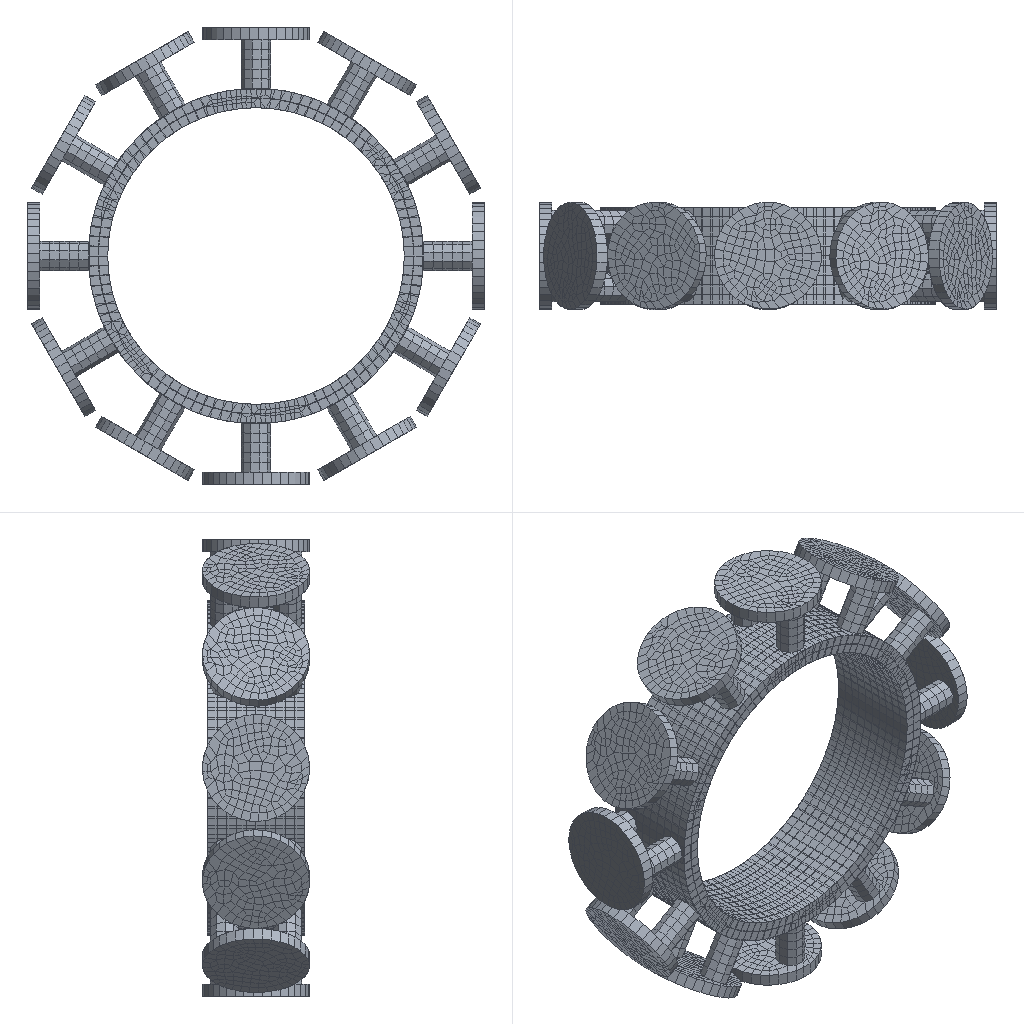Simulation study | abaqus
Set-up summary:
category,name,step,type,value,unit,region
solver,abaqus
solver,version,,,Abaqus/Standard 2020
units,not stated in the deck,,not stated
analysis,deck,,static,static
load_step,Step-1,Step-1,static
load_step,requested,,,1
mesh,nodes,,,21948
mesh,elements,,,16928
element_type,S4R,,shell,11811
element_type,C3D8R,,solid,5117
load,load commands in deck,,count,12
bc,support commands in deck,,count,5
material,CON,,in results
material,FRP,,in results
material,MATERIAL-3,,in results
check,setup vs results,,match,"per instance, exact: element labels, types and connectivity; labels of the nodes the elements use; coordinates of those nodes at SINGLE_PRECISION in 18 of 19 instance(s)"
Abaqus input file, long lists of numbers shortened:
*Heading
** Job name: Job-2 Model name: Model-1-Copy2
** Generated by: Abaqus/CAE 2020
*Preprint, echo=NO, model=NO, history=NO, contact=NO
**
** PARTS
**
*Part, name=con
*Node
      1,         610.,   1219.589,           0.
      2,         650.,   1219.589,           0.
** (916 more lines like these left out)
*Element, type=C3D8R
  1,  10,  11,  14,  13,   1,   2,   5,   4
  2,  11,  12,  15,  14,   2,   3,   6,   5
** (406 more lines like these left out)
*Nset, nset=Set-1, generate
   1,  918,    1
*Elset, elset=Set-1, generate
   1,  408,    1
** Section: con
*Solid Section, elset=Set-1, material=con
,
*End Part
**
*Part, name=frp
*Node
      1,   666.024,    1000.002,           0.
      2,   666.024,    1160.002,           0.
** (8318 more lines like these left out)
*Element, type=S4R
   1,   48,   41,    6,    1
   2,   41,   42,    7,    6
** (8318 more lines like these left out)
*Nset, nset=Set-3, generate
    1,  8320,     1
*Elset, elset=Set-3, generate
    1,  8320,     1
** Section: Section-1
*Shell Section, elset=Set-3, material=frp
7., 5
*End Part
**
*Part, name=gangban
*Node
      1,         610.,   1059.589,           0.
      2,         610.,   979.589,           0.
** (3081 more lines like these left out)
*Element, type=S4R
  1,    1,   13, 1241,  108
  2,   13,   14, 1242, 1241
** (3489 more lines like these left out)
*Nset, nset=Set-3, generate
    1,  3083,     1
*Elset, elset=Set-3, generate
    1,  3491,     1
** Section: Section-1
*Shell Section, elset=Set-3, material=frp
7., 5
*End Part
**
*Part, name=m1
*Node
      1,         890.,   1007.07,  -46.852
      2,   688.407,   1007.07,  -46.852
** (478 more lines like these left out)
*Element, type=C3D8R
 1, 434, 437, 435, 433, 114, 117, 115, 113
 2, 438, 434, 433, 436, 118, 114, 113, 116
** (239 more lines like these left out)
*Nset, nset=Set-1, generate
   1,  480,    1
*Elset, elset=Set-1, generate
   1,  241,    1
** Section: m
*Solid Section, elset=Set-1, material=Material-3
,
*End Part
**
*Part, name=m2
*Node
      1,   747.337,   1007.07,  -485.575
      2,   572.752,   1007.07,   -384.779
** (516 more lines like these left out)
*Element, type=C3D8R
 1, 119,  12,  11, 120, 453, 130, 129, 454
 2, 114,  10,   9, 121, 448, 128, 127, 455
** (273 more lines like these left out)
*Nset, nset=Set-3, generate
   1,  518,    1
*Elset, elset=Set-3, generate
   1,  275,    1
** Section: m
*Solid Section, elset=Set-3, material=Material-3
,
*End Part
**
*Part, name=m3
*Node
      1,   404.425,   1007.07,   -794.189
      2,   303.629,   1007.07,  -619.604
** (537 more lines like these left out)
*Element, type=C3D8R
 1, 119,  12,  11, 120, 462, 130, 129, 463
 2, 114,  10,   9, 121, 457, 128, 127, 464
** (291 more lines like these left out)
*Nset, nset=Set-1, generate
   1,  539,    1
*Elset, elset=Set-1, generate
   1,  293,    1
** Section: m
*Solid Section, elset=Set-1, material=Material-3
,
*End Part
**
*Part, name=m4
*Node
      1,  -46.852,   1007.07,        -890.
      2,  -46.852,   1007.07,  -688.407
** (478 more lines like these left out)
*Element, type=C3D8R
 1, 434, 437, 435, 433, 114, 117, 115, 113
 2, 438, 434, 433, 436, 118, 114, 113, 116
** (239 more lines like these left out)
*Nset, nset=Set-1, generate
   1,  480,    1
*Elset, elset=Set-1, generate
   1,  241,    1
** Section: m
*Solid Section, elset=Set-1, material=Material-3
,
*End Part
**
*Part, name=m5
*Node
      1,  -485.575,   1007.07,  -747.337
      2,   -384.779,   1007.07,  -572.752
** (487 more lines like these left out)
*Element, type=C3D8R
 1, 430, 123, 124, 434, 113,   8,   9, 117
 2, 432, 437, 433, 431, 115, 120, 116, 114
** (251 more lines like these left out)
*Nset, nset=Set-1, generate
   1,  489,    1
*Elset, elset=Set-1, generate
   1,  253,    1
** Section: m
*Solid Section, elset=Set-1, material=Material-3
,
*End Part
**
*Part, name=m6
*Node
      1,   -794.189,   1007.07,  -404.425
      2,  -619.604,   1007.07,  -303.629
** (466 more lines like these left out)
*Element, type=C3D8R
 1, 429, 118, 119, 120, 113,   8,   9,  10
 2, 125, 431, 430, 124,  15, 115, 114,  14
** (228 more lines like these left out)
*Nset, nset=Set-1, generate
   1,  468,    1
*Elset, elset=Set-1, generate
   1,  230,    1
** Section: m
*Solid Section, elset=Set-1, material=Material-3
,
*End Part
**
*Part, name=m7
*Node
      1,        -890.,   1007.07,   46.852
      2,  -688.407,   1007.07,   46.852
** (462 more lines like these left out)
*Element, type=C3D8R
 1, 118, 119, 427, 425,   8,   9, 115, 113
 2, 428, 426, 425, 427, 116, 114, 113, 115
** (226 more lines like these left out)
*Nset, nset=Set-1, generate
   1,  464,    1
*Elset, elset=Set-1, generate
   1,  228,    1
** Section: m
*Solid Section, elset=Set-1, material=Material-3
,
*End Part
**
*Part, name=m8
*Node
      1,  -747.337,   1007.07,   485.575
      2,  -572.752,   1007.07,    384.779
** (516 more lines like these left out)
*Element, type=C3D8R
 1, 119,  12,  11, 120, 453, 130, 129, 454
 2,  10,   9, 121, 114, 128, 127, 455, 448
** (273 more lines like these left out)
*Nset, nset=Set-1, generate
   1,  518,    1
*Elset, elset=Set-1, generate
   1,  275,    1
** Section: m
*Solid Section, elset=Set-1, material=Material-3
,
*End Part
**
*Part, name=m9
*Node
      1,  -404.425,   1007.07,    794.189
      2,  -303.629,   1007.07,   619.604
** (468 more lines like these left out)
*Element, type=C3D8R
 1, 423, 120, 121, 426, 113,   8,   9, 116
 2, 428, 426, 123, 124, 118, 116,  11,  12
** (234 more lines like these left out)
*Nset, nset=Set-1, generate
   1,  470,    1
*Elset, elset=Set-1, generate
   1,  236,    1
** Section: m
*Solid Section, elset=Set-1, material=Material-3
,
*End Part
**
*Part, name=m10
*Node
      1,   46.852,   1007.07,         890.
      2,   46.852,   1007.07,   688.407
** (541 more lines like these left out)
*Element, type=C3D8R
 1, 113, 123, 119, 120, 460, 470, 466, 467
 2, 114,  10,   9, 121, 461, 128, 127, 468
** (293 more lines like these left out)
*Nset, nset=Set-1, generate
   1,  543,    1
*Elset, elset=Set-1, generate
   1,  295,    1
** Section: m
*Solid Section, elset=Set-1, material=Material-3
,
*End Part
**
*Part, name=m11
*Node
      1,   485.575,   1007.07,   747.337
      2,    384.779,   1007.07,   572.752
** (516 more lines like these left out)
*Element, type=C3D8R
 1, 119,  12,  11, 120, 453, 130, 129, 454
 2, 114,  10,   9, 121, 448, 128, 127, 455
** (273 more lines like these left out)
*Nset, nset=Set-1, generate
   1,  518,    1
*Elset, elset=Set-1, generate
   1,  275,    1
** Section: m
*Solid Section, elset=Set-1, material=Material-3
,
*End Part
**
*Part, name=m12
*Node
      1,    794.189,   1007.07,   404.425
      2,   619.604,   1007.07,   303.629
** (466 more lines like these left out)
*Element, type=C3D8R
 1, 421, 120, 121, 424, 113,   8,   9, 116
 2, 426, 424, 123, 124, 118, 116,  11,  12
** (233 more lines like these left out)
*Nset, nset=Set-1, generate
   1,  468,    1
*Elset, elset=Set-1, generate
   1,  235,    1
** Section: m
*Solid Section, elset=Set-1, material=Material-3
,
*End Part
**
**
** ASSEMBLY
**
*Assembly, name=Assembly
**
*Instance, name=con-1, part=con
*End Instance
**
*Instance, name=frp-1, part=frp
*End Instance
**
*Instance, name=gangban-1, part=gangban
*End Instance
**
*Instance, name=con-1-lin-1-2, part=con
          0.,         -80.,           0.
*End Instance
**
*Instance, name=con-1-lin-1-3, part=con
          0.,        -160.,           0.
*End Instance
**
*Instance, name=con-1-lin-1-4, part=con
          0.,        -240.,           0.
*End Instance
**
*Instance, name=con-1-lin-1-5, part=con
          0.,        -320.,           0.
*End Instance
**
*Instance, name=m1-1, part=m1
*End Instance
**
*Instance, name=m2-1, part=m2
*End Instance
**
*Instance, name=m3-1, part=m3
*End Instance
**
*Instance, name=m4-1, part=m4
*End Instance
**
*Instance, name=m5-1, part=m5
*End Instance
**
*Instance, name=m6-1, part=m6
*End Instance
**
*Instance, name=m7-1, part=m7
*End Instance
**
*Instance, name=m8-1, part=m8
*End Instance
**
*Instance, name=m9-1, part=m9
*End Instance
**
*Instance, name=m10-1, part=m10
*End Instance
**
*Instance, name=m11-1, part=m11
*End Instance
**
*Instance, name=m12-1, part=m12
*End Instance
**
*Node
      1,         470.,   1099.589,   814.064
*Node
      2,   814.064,   1099.589,         470.
*Node
      3,         940.,   1099.589, 1.34711146e-14
*Node
      4,   814.064,   1099.589,        -470.
*Node
      5,         470.,   1099.589,  -814.064
*Node
      6, 7.10295131e-14,   1099.589,        -940.
*Node
      7,        -470.,   1099.589,  -814.064
*Node
      8,  -814.064,   1099.589,        -470.
*Node
      9,        -940.,   1099.589, -1.28587909e-13
*Node
     10,  -814.064,   1099.589,         470.
*Node
     11,        -470.,   1099.589,   814.064
*Node
     12, -1.86146319e-13,   1099.589,         940.
*Node
     13,           0.,   1059.589, -3.73517271e-14
*Nset, nset=Set-3, instance=con-1
   7,   8,   9,  16,  17,  18,  25,  26,  27,  34,  35,  36,  43,  44,  45,  52
  53,  54,  61,  62,  63,  70,  71,  72,  79,  80,  81,  88,  89,  90,  97,  98
** (18 more lines like these left out)
*Elset, elset=Set-3, instance=con-1
   3,   4,   7,   8,  11,  12,  15,  16,  19,  20,  23,  24,  27,  28,  31,  32
  35,  36,  39,  40,  43,  44,  47,  48,  51,  52,  55,  56,  59,  60,  63,  64
** (11 more lines like these left out)
*Nset, nset=Set-4, instance=m1-1
   4,   5,  34,  35,  36,  37,  38,  39,  40,  41,  42,  43,  44,  45,  46,  47
  48,  49,  50,  51,  52,  53,  54,  55,  56,  57,  58,  59,  60,  61,  62,  63
** (3 more lines like these left out)
*Nset, nset=Set-4, instance=m2-1
   4,   5,  34,  35,  36,  37,  38,  39,  40,  41,  42,  43,  44,  45,  46,  47
  48,  49,  50,  51,  52,  53,  54,  55,  56,  57,  58,  59,  60,  61,  62,  63
** (3 more lines like these left out)
*Nset, nset=Set-4, instance=m4-1
   4,   5,  34,  35,  36,  37,  38,  39,  40,  41,  42,  43,  44,  45,  46,  47
  48,  49,  50,  51,  52,  53,  54,  55,  56,  57,  58,  59,  60,  61,  62,  63
** (3 more lines like these left out)
*Nset, nset=Set-4, instance=m6-1
   4,   5,  34,  35,  36,  37,  38,  39,  40,  41,  42,  43,  44,  45,  46,  47
  48,  49,  50,  51,  52,  53,  54,  55,  56,  57,  58,  59,  60,  61,  62,  63
** (3 more lines like these left out)
*Nset, nset=Set-4, instance=m10-1
   4,   5,  34,  35,  36,  37,  38,  39,  40,  41,  42,  43,  44,  45,  46,  47
  48,  49,  50,  51,  52,  53,  54,  55,  56,  57,  58,  59,  60,  61,  62,  63
** (3 more lines like these left out)
*Nset, nset=Set-4, instance=m8-1
   4,   5,  34,  35,  36,  37,  38,  39,  40,  41,  42,  43,  44,  45,  46,  47
  48,  49,  50,  51,  52,  53,  54,  55,  56,  57,  58,  59,  60,  61,  62,  63
** (3 more lines like these left out)
*Nset, nset=Set-4, instance=m12-1
   4,   5,  34,  35,  36,  37,  38,  39,  40,  41,  42,  43,  44,  45,  46,  47
  48,  49,  50,  51,  52,  53,  54,  55,  56,  57,  58,  59,  60,  61,  62,  63
** (3 more lines like these left out)
*Nset, nset=Set-4, instance=m3-1
   4,   5,  34,  35,  36,  37,  38,  39,  40,  41,  42,  43,  44,  45,  46,  47
  48,  49,  50,  51,  52,  53,  54,  55,  56,  57,  58,  59,  60,  61,  62,  63
** (3 more lines like these left out)
*Nset, nset=Set-4, instance=m7-1
   4,   5,  34,  35,  36,  37,  38,  39,  40,  41,  42,  43,  44,  45,  46,  47
  48,  49,  50,  51,  52,  53,  54,  55,  56,  57,  58,  59,  60,  61,  62,  63
** (3 more lines like these left out)
*Nset, nset=Set-4, instance=m11-1
   4,   5,  34,  35,  36,  37,  38,  39,  40,  41,  42,  43,  44,  45,  46,  47
  48,  49,  50,  51,  52,  53,  54,  55,  56,  57,  58,  59,  60,  61,  62,  63
** (3 more lines like these left out)
*Nset, nset=Set-4, instance=m5-1
   4,   5,  34,  35,  36,  37,  38,  39,  40,  41,  42,  43,  44,  45,  46,  47
  48,  49,  50,  51,  52,  53,  54,  55,  56,  57,  58,  59,  60,  61,  62,  63
** (3 more lines like these left out)
*Nset, nset=Set-4, instance=m9-1
   4,   5,  34,  35,  36,  37,  38,  39,  40,  41,  42,  43,  44,  45,  46,  47
  48,  49,  50,  51,  52,  53,  54,  55,  56,  57,  58,  59,  60,  61,  62,  63
** (3 more lines like these left out)
*Elset, elset=Set-4, instance=m1-1
  77,  80,  82,  83,  84,  86,  88,  90,  91,  92,  98,  99, 100, 104, 105, 106
 107, 109, 111, 112, 113, 116, 118, 122, 129, 130, 131, 132, 133, 134, 136, 137
** (1 more lines like these left out)
*Elset, elset=Set-4, instance=m2-1
 101, 106, 107, 108, 109, 110, 111, 112, 113, 115, 117, 122, 123, 130, 131, 132
 133, 134, 138, 141, 143, 147, 153, 154, 156, 157, 158, 159, 160, 161, 164, 165
** (1 more lines like these left out)
*Elset, elset=Set-4, instance=m4-1
  77,  80,  82,  83,  84,  87,  89,  91,  92,  93,  99, 100, 101, 104, 105, 106
 107, 109, 111, 112, 113, 116, 117, 121, 129, 130, 131, 132, 133, 134, 136, 137
** (1 more lines like these left out)
*Elset, elset=Set-4, instance=m6-1
  52,  53,  61,  62,  66,  67,  68,  70,  71,  72,  73,  74,  76,  80,  84,  88
  89,  92,  93,  94,  97, 101, 107, 112, 113, 114, 117, 118, 119, 121, 122, 124
** (1 more lines like these left out)
*Elset, elset=Set-4, instance=m10-1
 103, 111, 112, 114, 115, 116, 118, 120, 123, 124, 126, 131, 133, 137, 138, 139
 140, 142, 145, 148, 150, 153, 160, 161, 162, 163, 164, 165, 166, 167, 168, 170
** (1 more lines like these left out)
*Elset, elset=Set-4, instance=m8-1
 100, 105, 106, 107, 108, 109, 110, 111, 112, 113, 115, 120, 121, 122, 130, 131
 133, 134, 138, 142, 145, 153, 154, 155, 156, 157, 158, 159, 161, 162, 165, 166
** (1 more lines like these left out)
*Elset, elset=Set-4, instance=m12-1
  62,  63,  71,  75,  76,  77,  79,  80,  81,  82,  83,  85,  89,  91,  94,  97
  98, 101, 102, 103, 106, 110, 115, 122, 123, 124, 125, 126, 129, 130, 134, 135
** (1 more lines like these left out)
*Elset, elset=Set-4, instance=m3-1
  95,  96, 104, 109, 110, 111, 113, 114, 115, 116, 118, 123, 124, 127, 131, 132
 135, 136, 138, 141, 145, 149, 153, 158, 159, 161, 162, 163, 165, 166, 168, 169
** (1 more lines like these left out)
*Elset, elset=Set-4, instance=m7-1
  67,  70,  72,  73,  74,  77,  79,  81,  82,  83,  89,  90,  91,  94,  95,  96
  97,  99, 100, 101, 102, 105, 106, 111, 118, 119, 120, 122, 123, 124, 126, 127
** (1 more lines like these left out)
*Elset, elset=Set-4, instance=m11-1
 101, 106, 107, 109, 110, 111, 112, 113, 115, 117, 122, 123, 124, 131, 132, 133
 134, 138, 141, 145, 147, 152, 153, 154, 155, 157, 159, 160, 161, 162, 165, 166
** (1 more lines like these left out)
*Elset, elset=Set-4, instance=m5-1
  86,  91,  92,  93,  94,  96,  97,  98, 100, 102, 106, 115, 116, 117, 118, 119
 121, 124, 126, 133, 137, 138, 140, 141, 142, 143, 144, 145, 146, 147, 151, 152
** (1 more lines like these left out)
*Elset, elset=Set-4, instance=m9-1
  62,  63,  71,  75,  76,  77,  78,  80,  81,  82,  83,  85,  87,  91,  93,  99
 100, 103, 104, 105, 108, 112, 117, 120, 124, 125, 126, 127, 130, 131, 135, 136
** (1 more lines like these left out)
*Nset, nset=Set-30
 13,
*Nset, nset=b_Set-5, instance=m11-1, generate
   1,  518,    1
*Elset, elset=b_Set-5, instance=m11-1, generate
   1,  275,    1
*Nset, nset=b_Set-7, instance=m12-1, generate
   1,  468,    1
*Elset, elset=b_Set-7, instance=m12-1, generate
   1,  235,    1
*Nset, nset=b_Set-9, instance=m1-1, generate
   1,  480,    1
*Elset, elset=b_Set-9, instance=m1-1, generate
   1,  241,    1
*Nset, nset=b_Set-11, instance=m2-1, generate
   1,  518,    1
*Elset, elset=b_Set-11, instance=m2-1, generate
   1,  275,    1
*Nset, nset=b_Set-13, instance=m3-1, generate
   1,  539,    1
*Elset, elset=b_Set-13, instance=m3-1, generate
   1,  293,    1
*Nset, nset=b_Set-15, instance=m4-1, generate
   1,  480,    1
*Elset, elset=b_Set-15, instance=m4-1, generate
   1,  241,    1
*Nset, nset=b_Set-17, instance=m5-1, generate
   1,  489,    1
*Elset, elset=b_Set-17, instance=m5-1, generate
   1,  253,    1
*Nset, nset=b_Set-19, instance=m6-1, generate
   1,  468,    1
*Elset, elset=b_Set-19, instance=m6-1, generate
   1,  230,    1
*Nset, nset=b_Set-21, instance=m7-1, generate
   1,  464,    1
*Elset, elset=b_Set-21, instance=m7-1, generate
   1,  228,    1
*Nset, nset=b_Set-23, instance=m8-1, generate
   1,  518,    1
*Elset, elset=b_Set-23, instance=m8-1, generate
   1,  275,    1
*Nset, nset=b_Set-25, instance=m9-1, generate
   1,  470,    1
*Elset, elset=b_Set-25, instance=m9-1, generate
   1,  236,    1
*Nset, nset=b_Set-27, instance=m10-1, generate
   1,  543,    1
*Elset, elset=b_Set-27, instance=m10-1, generate
   1,  295,    1
*Nset, nset=m_Set-1, instance=frp-1, generate
    1,  8320,     1
*Elset, elset=m_Set-1, instance=frp-1, generate
    1,  8320,     1
*Nset, nset=m_Set-29
 13,
*Nset, nset=s_Set-1, instance=con-1, generate
   1,  918,    1
*Nset, nset=s_Set-1, instance=con-1-lin-1-2, generate
   1,  918,    1
*Nset, nset=s_Set-1, instance=con-1-lin-1-3, generate
   1,  918,    1
*Nset, nset=s_Set-1, instance=con-1-lin-1-5, generate
   1,  918,    1
*Nset, nset=s_Set-1, instance=con-1-lin-1-4, generate
   1,  918,    1
*Elset, elset=s_Set-1, instance=con-1, generate
   1,  408,    1
*Elset, elset=s_Set-1, instance=con-1-lin-1-2, generate
   1,  408,    1
*Elset, elset=s_Set-1, instance=con-1-lin-1-3, generate
   1,  408,    1
*Elset, elset=s_Set-1, instance=con-1-lin-1-5, generate
   1,  408,    1
*Elset, elset=s_Set-1, instance=con-1-lin-1-4, generate
   1,  408,    1
*Nset, nset=_PickedSet98, internal
 1,
*Nset, nset=_PickedSet100, internal
 2,
*Nset, nset=_PickedSet102, internal
 3,
*Nset, nset=_PickedSet104, internal
 4,
*Nset, nset=_PickedSet106, internal
 5,
*Nset, nset=_PickedSet108, internal
 6,
*Nset, nset=_PickedSet110, internal
 7,
*Nset, nset=_PickedSet112, internal
 8,
*Nset, nset=_PickedSet114, internal
 9,
*Nset, nset=_PickedSet116, internal
 10,
*Nset, nset=_PickedSet118, internal
 11,
*Nset, nset=_PickedSet120, internal
 12,
*Elset, elset=_Surf-1_S1, internal, instance=m10-1, generate
  81,  214,    1
*Elset, elset=_Surf-1_S2, internal, instance=m10-1, generate
 215,  230,    1
*Surface, type=ELEMENT, name=Surf-1
_Surf-1_S1, S1
_Surf-1_S2, S2
*Elset, elset=_Surf-2_S2, internal, instance=m9-1
  51,  52,  53,  54,  55,  56,  57,  58,  59,  60, 177, 178, 179, 180, 181, 182
 183, 184, 185, 186
*Elset, elset=_Surf-2_S1, internal, instance=m9-1, generate
  61,  176,    1
*Surface, type=ELEMENT, name=Surf-2
_Surf-2_S2, S2
_Surf-2_S1, S1
*Elset, elset=_Surf-3_S1, internal, instance=m8-1, generate
  81,  209,    1
*Elset, elset=_Surf-3_S2, internal, instance=m8-1, generate
 210,  225,    1
*Surface, type=ELEMENT, name=Surf-3
_Surf-3_S1, S1
_Surf-3_S2, S2
*Elset, elset=_Surf-4_S2, internal, instance=m7-1
  41,  42,  43,  44,  45,  46,  47,  48,  49,  50, 171, 172, 173, 174, 175, 176
 177, 178
*Elset, elset=_Surf-4_S1, internal, instance=m7-1, generate
  51,  170,    1
*Surface, type=ELEMENT, name=Surf-4
_Surf-4_S2, S2
_Surf-4_S1, S1
*Elset, elset=_Surf-5_S2, internal, instance=m6-1
  41,  42,  43,  44,  45,  46,  47,  48,  49,  50, 173, 174, 175, 176, 177, 178
 179, 180
*Elset, elset=_Surf-5_S1, internal, instance=m6-1, generate
  51,  172,    1
*Surface, type=ELEMENT, name=Surf-5
_Surf-5_S2, S2
_Surf-5_S1, S1
*Elset, elset=_Surf-6_S2, internal, instance=m5-1
  66,  67,  68,  69,  70,  71,  72,  73,  74,  75, 191, 192, 193, 194, 195, 196
 197, 198, 199, 200, 201, 202, 203
*Elset, elset=_Surf-6_S1, internal, instance=m5-1, generate
  76,  190,    1
*Surface, type=ELEMENT, name=Surf-6
_Surf-6_S2, S2
_Surf-6_S1, S1
*Elset, elset=_Surf-7_S2, internal, instance=m4-1
  51,  52,  53,  54,  55,  56,  57,  58,  59,  60, 182, 183, 184, 185, 186, 187
 188, 189, 190, 191
*Elset, elset=_Surf-7_S1, internal, instance=m4-1, generate
  61,  181,    1
*Surface, type=ELEMENT, name=Surf-7
_Surf-7_S2, S2
_Surf-7_S1, S1
*Elset, elset=_Surf-8_S1, internal, instance=m3-1, generate
  81,  212,    1
*Elset, elset=_Surf-8_S2, internal, instance=m3-1, generate
 213,  228,    1
*Surface, type=ELEMENT, name=Surf-8
_Surf-8_S1, S1
_Surf-8_S2, S2
*Elset, elset=_Surf-9_S1, internal, instance=m2-1, generate
  81,  209,    1
*Elset, elset=_Surf-9_S2, internal, instance=m2-1, generate
 210,  225,    1
*Surface, type=ELEMENT, name=Surf-9
_Surf-9_S1, S1
_Surf-9_S2, S2
*Elset, elset=_Surf-10_S2, internal, instance=m1-1
  51,  52,  53,  54,  55,  56,  57,  58,  59,  60, 182, 183, 184, 185, 186, 187
 188, 189, 190, 191
*Elset, elset=_Surf-10_S1, internal, instance=m1-1, generate
  61,  181,    1
*Surface, type=ELEMENT, name=Surf-10
_Surf-10_S2, S2
_Surf-10_S1, S1
*Elset, elset=_Surf-11_S2, internal, instance=m12-1
  51,  52,  53,  54,  55,  56,  57,  58,  59,  60, 176, 177, 178, 179, 180, 181
 182, 183, 184, 185
*Elset, elset=_Surf-11_S1, internal, instance=m12-1, generate
  61,  175,    1
*Surface, type=ELEMENT, name=Surf-11
_Surf-11_S2, S2
_Surf-11_S1, S1
*Elset, elset=_Surf-12_S1, internal, instance=m11-1, generate
  81,  209,    1
*Elset, elset=_Surf-12_S2, internal, instance=m11-1, generate
 210,  225,    1
*Surface, type=ELEMENT, name=Surf-12
_Surf-12_S1, S1
_Surf-12_S2, S2
*Elset, elset=_m_Surf-15_S3, internal, instance=con-1
   1,   2,   5,   6,   9,  10,  13,  14,  17,  18,  21,  22,  25,  26,  29,  30
  33,  34,  37,  38,  41,  42,  45,  46,  49,  50,  53,  54,  57,  58,  61,  62
** (11 more lines like these left out)
*Elset, elset=_m_Surf-15_S3, internal, instance=con-1-lin-1-2
   1,   2,   5,   6,   9,  10,  13,  14,  17,  18,  21,  22,  25,  26,  29,  30
  33,  34,  37,  38,  41,  42,  45,  46,  49,  50,  53,  54,  57,  58,  61,  62
** (11 more lines like these left out)
*Elset, elset=_m_Surf-15_S3, internal, instance=con-1-lin-1-3
   1,   2,   5,   6,   9,  10,  13,  14,  17,  18,  21,  22,  25,  26,  29,  30
  33,  34,  37,  38,  41,  42,  45,  46,  49,  50,  53,  54,  57,  58,  61,  62
** (11 more lines like these left out)
*Elset, elset=_m_Surf-15_S3, internal, instance=con-1-lin-1-5
   1,   2,   5,   6,   9,  10,  13,  14,  17,  18,  21,  22,  25,  26,  29,  30
  33,  34,  37,  38,  41,  42,  45,  46,  49,  50,  53,  54,  57,  58,  61,  62
** (11 more lines like these left out)
*Elset, elset=_m_Surf-15_S3, internal, instance=con-1-lin-1-4
   1,   2,   5,   6,   9,  10,  13,  14,  17,  18,  21,  22,  25,  26,  29,  30
  33,  34,  37,  38,  41,  42,  45,  46,  49,  50,  53,  54,  57,  58,  61,  62
** (11 more lines like these left out)
*Elset, elset=_m_Surf-15_S6, internal, instance=con-1, generate
   1,  407,    2
*Elset, elset=_m_Surf-15_S6, internal, instance=con-1-lin-1-2, generate
   1,  407,    2
*Elset, elset=_m_Surf-15_S6, internal, instance=con-1-lin-1-3, generate
   1,  407,    2
*Elset, elset=_m_Surf-15_S6, internal, instance=con-1-lin-1-5, generate
   1,  407,    2
*Elset, elset=_m_Surf-15_S6, internal, instance=con-1-lin-1-4, generate
   1,  407,    2
*Elset, elset=_m_Surf-15_S5, internal, instance=con-1
   3,   4,   7,   8,  11,  12,  15,  16,  19,  20,  23,  24,  27,  28,  31,  32
  35,  36,  39,  40,  43,  44,  47,  48,  51,  52,  55,  56,  59,  60,  63,  64
** (11 more lines like these left out)
*Elset, elset=_m_Surf-15_S5, internal, instance=con-1-lin-1-2
   3,   4,   7,   8,  11,  12,  15,  16,  19,  20,  23,  24,  27,  28,  31,  32
  35,  36,  39,  40,  43,  44,  47,  48,  51,  52,  55,  56,  59,  60,  63,  64
** (11 more lines like these left out)
*Elset, elset=_m_Surf-15_S5, internal, instance=con-1-lin-1-3
   3,   4,   7,   8,  11,  12,  15,  16,  19,  20,  23,  24,  27,  28,  31,  32
  35,  36,  39,  40,  43,  44,  47,  48,  51,  52,  55,  56,  59,  60,  63,  64
** (11 more lines like these left out)
*Elset, elset=_m_Surf-15_S5, internal, instance=con-1-lin-1-5
   3,   4,   7,   8,  11,  12,  15,  16,  19,  20,  23,  24,  27,  28,  31,  32
  35,  36,  39,  40,  43,  44,  47,  48,  51,  52,  55,  56,  59,  60,  63,  64
** (11 more lines like these left out)
*Elset, elset=_m_Surf-15_S5, internal, instance=con-1-lin-1-4
   3,   4,   7,   8,  11,  12,  15,  16,  19,  20,  23,  24,  27,  28,  31,  32
  35,  36,  39,  40,  43,  44,  47,  48,  51,  52,  55,  56,  59,  60,  63,  64
** (11 more lines like these left out)
*Elset, elset=_m_Surf-15_S4, internal, instance=con-1, generate
   2,  408,    2
*Elset, elset=_m_Surf-15_S4, internal, instance=con-1-lin-1-2, generate
   2,  408,    2
*Elset, elset=_m_Surf-15_S4, internal, instance=con-1-lin-1-3, generate
   2,  408,    2
*Elset, elset=_m_Surf-15_S4, internal, instance=con-1-lin-1-5, generate
   2,  408,    2
*Elset, elset=_m_Surf-15_S4, internal, instance=con-1-lin-1-4, generate
   2,  408,    2
*Surface, type=ELEMENT, name=m_Surf-15
_m_Surf-15_S3, S3
_m_Surf-15_S6, S6
_m_Surf-15_S4, S4
_m_Surf-15_S5, S5
*Elset, elset=_m_Surf-17_SPOS, internal, instance=gangban-1
  193,  194,  195,  196,  197,  198,  199,  200,  201,  202,  203,  204,  205,  206,  207,  208
  209,  210,  211,  212,  213,  214,  215,  216,  217,  218,  219,  220,  221,  222,  223,  224
** (66 more lines like these left out)
*Surface, type=ELEMENT, name=m_Surf-17
_m_Surf-17_SPOS, SPOS
*Elset, elset=_s_Surf-14_SPOS, internal, instance=gangban-1, generate
 3017,  3491,     1
*Surface, type=ELEMENT, name=s_Surf-14
_s_Surf-14_SPOS, SPOS
*Elset, elset=_s_Surf-15_SNEG, internal, instance=gangban-1, generate
    1,  3491,     1
*Surface, type=ELEMENT, name=s_Surf-15
_s_Surf-15_SNEG, SNEG
*Elset, elset=_s_Surf-17_S2, internal, instance=m1-1, generate
 232,  241,    1
*Elset, elset=_s_Surf-17_S2, internal, instance=m2-1
  65,  66,  67,  68,  69,  70,  71,  72,  73,  74,  75,  76,  77,  78,  79,  80
 266, 267, 268, 269, 270, 271, 272, 273, 274, 275
*Elset, elset=_s_Surf-17_S2, internal, instance=m4-1, generate
 232,  241,    1
*Elset, elset=_s_Surf-17_S2, internal, instance=m6-1, generate
 221,  230,    1
*Elset, elset=_s_Surf-17_S2, internal, instance=m10-1
  65,  66,  67,  68,  69,  70,  71,  72,  73,  74,  75,  76,  77,  78,  79,  80
 283, 284, 285, 286, 287, 288, 289, 290, 291, 292, 293, 294, 295
*Elset, elset=_s_Surf-17_S2, internal, instance=m8-1
  65,  66,  67,  68,  69,  70,  71,  72,  73,  74,  75,  76,  77,  78,  79,  80
 266, 267, 268, 269, 270, 271, 272, 273, 274, 275
*Elset, elset=_s_Surf-17_S2, internal, instance=m12-1, generate
 226,  235,    1
*Elset, elset=_s_Surf-17_S2, internal, instance=m3-1
  65,  66,  67,  68,  69,  70,  71,  72,  73,  74,  75,  76,  77,  78,  79,  80
 281, 282, 283, 284, 285, 286, 287, 288, 289, 290, 291, 292, 293
*Elset, elset=_s_Surf-17_S2, internal, instance=m7-1, generate
 219,  228,    1
*Elset, elset=_s_Surf-17_S2, internal, instance=m11-1
  65,  66,  67,  68,  69,  70,  71,  72,  73,  74,  75,  76,  77,  78,  79,  80
 266, 267, 268, 269, 270, 271, 272, 273, 274, 275
*Elset, elset=_s_Surf-17_S2, internal, instance=m5-1, generate
 244,  253,    1
*Elset, elset=_s_Surf-17_S2, internal, instance=m9-1, generate
 227,  236,    1
*Elset, elset=_s_Surf-17_S1, internal, instance=m1-1, generate
 41,  50,   1
*Elset, elset=_s_Surf-17_S1, internal, instance=m4-1, generate
 41,  50,   1
*Elset, elset=_s_Surf-17_S1, internal, instance=m6-1, generate
 33,  40,   1
*Elset, elset=_s_Surf-17_S1, internal, instance=m12-1, generate
 41,  50,   1
*Elset, elset=_s_Surf-17_S1, internal, instance=m7-1, generate
 33,  40,   1
*Elset, elset=_s_Surf-17_S1, internal, instance=m5-1, generate
 53,  65,   1
*Elset, elset=_s_Surf-17_S1, internal, instance=m9-1, generate
 41,  50,   1
*Surface, type=ELEMENT, name=s_Surf-17
_s_Surf-17_S2, S2
_s_Surf-17_S1, S1
*Elset, elset=_shuchu_SPOS, internal, instance=gangban-1
  193,  194,  195,  196,  197,  198,  199,  200,  201,  202,  203,  204,  205,  206,  207,  208
  209,  210,  211,  212,  213,  214,  215,  216,  217,  218,  219,  220,  221,  222,  223,  224
** (66 more lines like these left out)
*Surface, type=ELEMENT, name=shuchu
_shuchu_SPOS, SPOS
** Constraint: Constraint-1
*Embedded Element, host elset=s_Set-1
m_Set-1
** Constraint: Constraint-2
*Rigid Body, ref node=_PickedSet98, elset=b_Set-5
** Constraint: Constraint-3
*Rigid Body, ref node=_PickedSet100, elset=b_Set-7
** Constraint: Constraint-4
*Rigid Body, ref node=_PickedSet102, elset=b_Set-9
** Constraint: Constraint-5
*Rigid Body, ref node=_PickedSet104, elset=b_Set-11
** Constraint: Constraint-6
*Rigid Body, ref node=_PickedSet106, elset=b_Set-13
** Constraint: Constraint-7
*Rigid Body, ref node=_PickedSet108, elset=b_Set-15
** Constraint: Constraint-8
*Rigid Body, ref node=_PickedSet110, elset=b_Set-17
** Constraint: Constraint-9
*Rigid Body, ref node=_PickedSet112, elset=b_Set-19
** Constraint: Constraint-10
*Rigid Body, ref node=_PickedSet114, elset=b_Set-21
** Constraint: Constraint-11
*Rigid Body, ref node=_PickedSet116, elset=b_Set-23
** Constraint: Constraint-12
*Rigid Body, ref node=_PickedSet118, elset=b_Set-25
** Constraint: Constraint-13
*Rigid Body, ref node=_PickedSet120, elset=b_Set-27
** Constraint: Constraint-15
*Tie, name=Constraint-15, adjust=yes
m_Surf-15, s_Surf-15
** Constraint: Constraint-SHUCHU
*Coupling, constraint name=Constraint-SHUCHU, ref node=m_Set-29, surface=s_Surf-14
*Kinematic
*End Assembly
*Amplitude, name=Amp-1
             0.,              0.,              1.,              1.
**
** MATERIALS
**
*Material, name=Material-3
*Density
 7.8e-09,
*Elastic
180000., 0.3
*Plastic
147.,0.
*Material, name=con
*Density
 2.2e-09,
*Elastic
35900., 0.22
*Plastic
30.,0.
*Material, name=frp
*Density
 1.5e-09,
*Elastic, type=ENGINEERING CONSTANTS
11810.,11200.,11810.,  0.24,  0.23,  0.23, 7800., 8900.
 8900.,
**
** INTERACTION PROPERTIES
**
*Surface Interaction, name=IntProp-1
1.,
*Friction, slip tolerance=0.005
 0.2,
*Surface Behavior, pressure-overclosure=HARD
**
** INTERACTIONS
**
** Interaction: Int-2
*Contact Pair, interaction=IntProp-1, type=SURFACE TO SURFACE, adjust=1.
m_Surf-17, s_Surf-17
** ----------------------------------------------------------------
**
** STEP: Step-1
**
*Step, name=Step-1, nlgeom=YES, inc=1000
*Static, stabilize=0.0002, allsdtol=0.05, continue=NO
0.01, 1., 1e-05, 1.
**
** BOUNDARY CONDITIONS
**
** Name: BC-2 Type: 位移/转角
*Boundary
Set-4, 2, 2
Set-4, 4, 4
Set-4, 5, 5
Set-4, 6, 6
** Name: BC-3 Type: 对称/反对称/完全固定
*Boundary
Set-30, ENCASTRE
**
** LOADS
**
** Name: Load-1   Type: Pressure
*Dsload, amplitude=Amp-1
Surf-1, P, 10.58
** Name: Load-2   Type: Pressure
*Dsload, amplitude=Amp-1
Surf-2, P, 10.837
** Name: Load-3   Type: Pressure
*Dsload, amplitude=Amp-1
Surf-3, P, 12.166
** Name: Load-4   Type: Pressure
*Dsload, amplitude=Amp-1
Surf-4, P, 11.26
** Name: Load-5   Type: Pressure
*Dsload, amplitude=Amp-1
Surf-5, P, 11.3
** Name: Load-6   Type: Pressure
*Dsload, amplitude=Amp-1
Surf-6, P, 10.7
** Name: Load-7   Type: Pressure
*Dsload, amplitude=Amp-1
Surf-7, P, 12.
** Name: Load-8   Type: Pressure
*Dsload, amplitude=Amp-1
Surf-8, P, 12.357
** Name: Load-9   Type: Pressure
*Dsload, amplitude=Amp-1
Surf-9, P, 13.05
** Name: Load-10   Type: Pressure
*Dsload, amplitude=Amp-1
Surf-10, P, 12.4
** Name: Load-11   Type: Pressure
*Dsload, amplitude=Amp-1
Surf-11, P, 11.837
** Name: Load-12   Type: Pressure
*Dsload, amplitude=Amp-1
Surf-12, P, 11.139
**
** OUTPUT REQUESTS
**
*Restart, write, number interval=1, time marks=NO
**
** FIELD OUTPUT: F-Output-1
**
*Output, field
*Node Output
CF, RF, RM, RT, U, V
*Element Output, directions=YES
E, LE, MISES, MISESMAX, MISESONLY, PE, PEEQ, S, SF, SSAVG
*Contact Output
CDISP, CSTRESS
**
** HISTORY OUTPUT: H-Output-1
**
*Output, history
*Node Output, nset=Set-30
RF1, RF3, U1, U3
*End Step
Results summary:
result,step,,completed,increments=11 time=1.0/1.0
result,analysis,,,static
result,last_loadstep,,,1
result,primary field,,,"U, UR"
result,reaction total,,FX,505869.656,model units
result,reaction total,,FY,-88.296,model units
result,reaction total,,FZ,-381952.219,model units